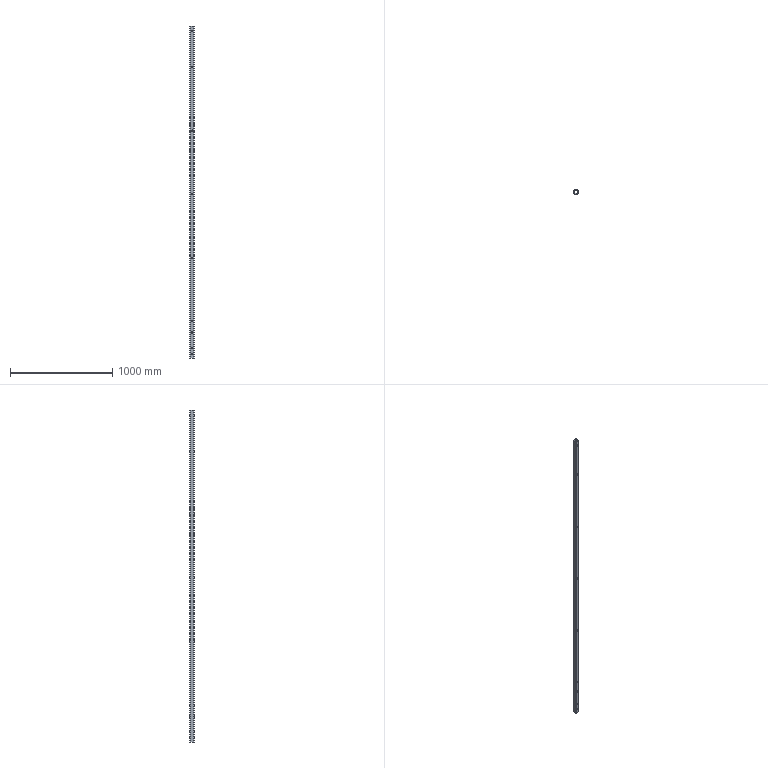Part | STEP file | IN-01-01-04-01 | 1 solid | 54 faces | box 40 x 40 x 3250 mm | volume 1322181 mm3 | cylinder 44 | plane 10 | commonest cylinder face diameters 12.2 x36 5.8 x4 11.6 x4